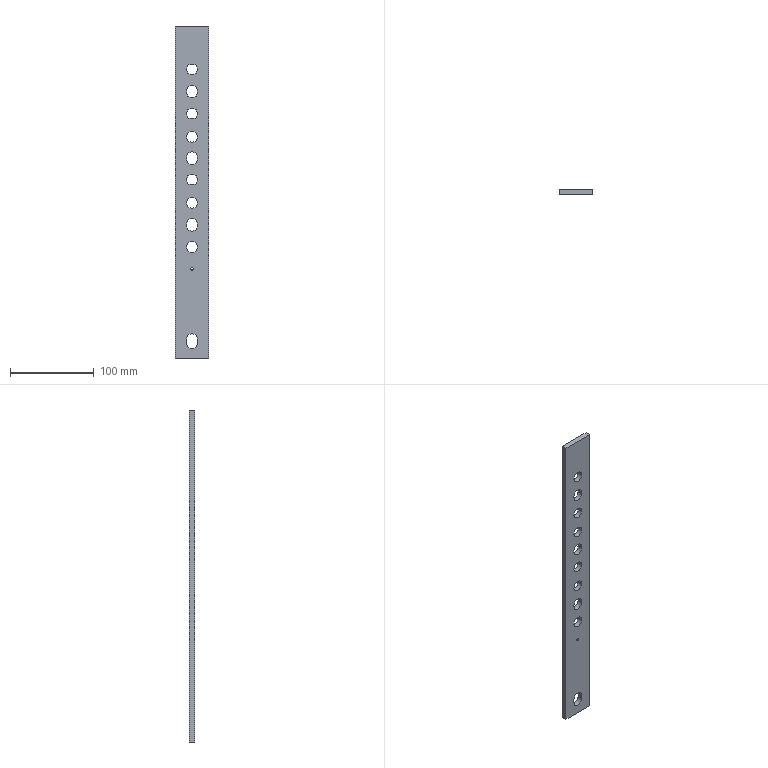Part | STEP file | 64586807 | 1 solid | 36 faces | box 40 x 6 x 397.5 mm | volume 86530 mm3 | cylinder 22 | plane 14 | commonest cylinder face diameters 13 x20 3.2 x2